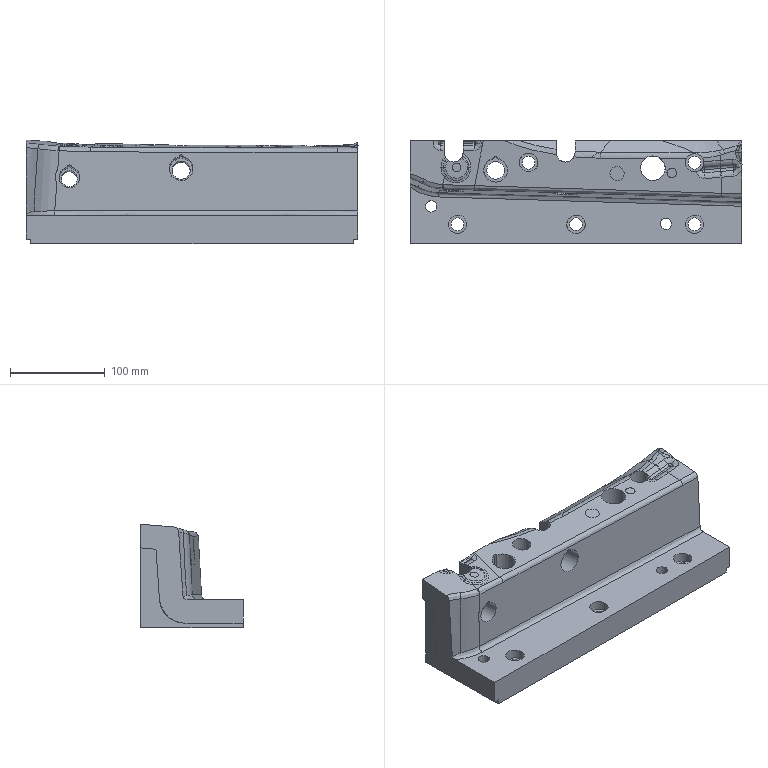Part | NX | features solid 2 | 1 solid | 139 faces | box 350 x 108 x 109.429 mm | volume 2317748 mm3 | spline 59 | cylinder 44 | plane 29 | sphere 5 | torus 1 | cone 1 | commonest cylinder face diameters 13.5 x5 19.5 x5 16 x4 4 x3 20 x3 12 x2